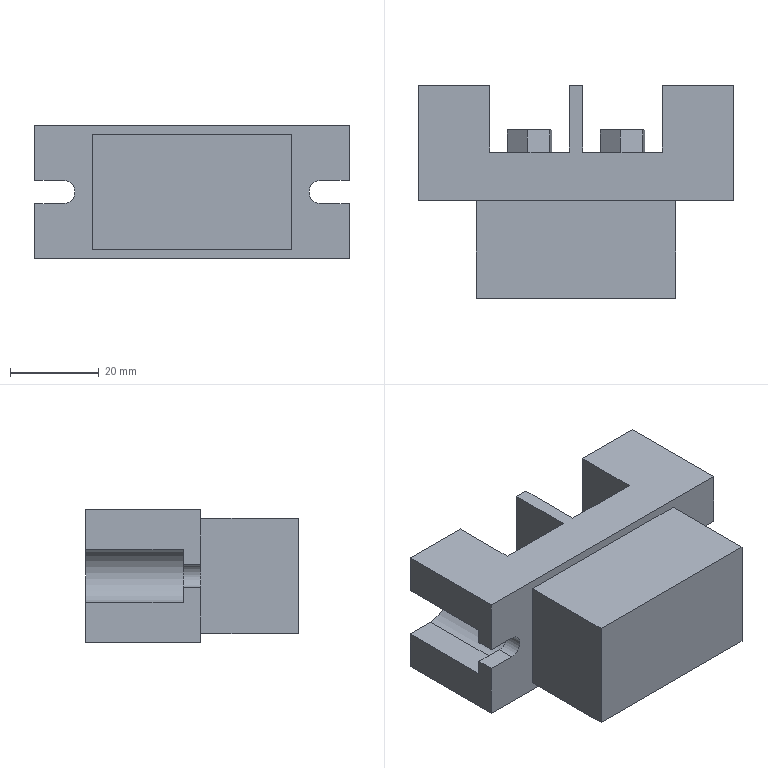Part | SolidWorks | features ICE 5, LPattern 2, Extrusion 1 | 1 solid | 49 faces | box 71 x 48 x 30 mm | volume 59444 mm3 | plane 45 | cylinder 4 | commonest cylinder face diameters 5.2 x2 12 x2
STEP:
#1=CARTESIAN_POINT('',(-19.5,11.,-15.));
#2=VERTEX_POINT('',#1);
#3=CARTESIAN_POINT('',(-19.5,11.,15.));
#4=VERTEX_POINT('',#3);
#5=CARTESIAN_POINT('',(-19.5,11.,-15.));
#6=DIRECTION('',(0.,0.,1.));
#7=VECTOR('',#6,1000.);
#8=LINE('',#5,#7);
#9=EDGE_CURVE('',#2,#4,#8,.T.);
#10=ORIENTED_EDGE('',*,*,#9,.T.);
#11=CARTESIAN_POINT('',(-1.5,11.,15.));
#12=VERTEX_POINT('',#11);
#13=CARTESIAN_POINT('',(-19.5,11.,15.));
#14=DIRECTION('',(1.,0.,0.));
#15=VECTOR('',#14,1000.);
#16=LINE('',#13,#15);
#17=EDGE_CURVE('',#4,#12,#16,.T.);
#18=ORIENTED_EDGE('',*,*,#17,.T.);
#19=CARTESIAN_POINT('',(-1.5,11.,-15.));
#20=VERTEX_POINT('',#19);
#21=CARTESIAN_POINT('',(-1.5,11.,-15.));
#22=DIRECTION('',(0.,0.,-1.));
#23=VECTOR('',#22,1000.);
#24=LINE('',#21,#23);
#25=EDGE_CURVE('',#12,#20,#24,.T.);
#26=ORIENTED_EDGE('',*,*,#25,.T.);
#27=CARTESIAN_POINT('',(-19.5,11.,-15.));
#28=DIRECTION('',(-1.,0.,0.));
#29=VECTOR('',#28,1000.);
#30=LINE('',#27,#29);
#31=EDGE_CURVE('',#20,#2,#30,.T.);
#32=ORIENTED_EDGE('',*,*,#31,.T.);
#33=EDGE_LOOP('',(#10,#18,#26,#32));
#34=FACE_OUTER_BOUND('',#33,.T.);
#35=CARTESIAN_POINT('',(-5.967,11.,3.196));
#36=VERTEX_POINT('',#35);
#37=CARTESIAN_POINT('',(-5.466,11.,-2.328));
#38=VERTEX_POINT('',#37);
#39=CARTESIAN_POINT('',(-5.967,11.,3.196));
#40=DIRECTION('',(0.09034,0.,-0.9959));
#41=VECTOR('',#40,1000.);
#42=LINE('',#39,#41);
#43=EDGE_CURVE('',#36,#38,#42,.T.);
#44=ORIENTED_EDGE('',*,*,#43,.F.);
#45=CARTESIAN_POINT('',(-11.001,11.,5.524));
#46=VERTEX_POINT('',#45);
#47=CARTESIAN_POINT('',(-11.001,11.,5.524));
#48=DIRECTION('',(0.9077,0.,-0.4197));
#49=VECTOR('',#48,1000.);
#50=LINE('',#47,#49);
#51=EDGE_CURVE('',#46,#36,#50,.T.);
#52=ORIENTED_EDGE('',*,*,#51,.F.);
#53=CARTESIAN_POINT('',(-15.534,11.,2.328));
#54=VERTEX_POINT('',#53);
#55=CARTESIAN_POINT('',(-15.534,11.,2.328));
#56=DIRECTION('',(0.8173,0.,0.5762));
#57=VECTOR('',#56,1000.);
#58=LINE('',#55,#57);
#59=EDGE_CURVE('',#54,#46,#58,.T.);
#60=ORIENTED_EDGE('',*,*,#59,.F.);
#61=CARTESIAN_POINT('',(-15.033,11.,-3.196));
#62=VERTEX_POINT('',#61);
#63=CARTESIAN_POINT('',(-15.033,11.,-3.196));
#64=DIRECTION('',(-0.09034,0.,0.9959));
#65=VECTOR('',#64,1000.);
#66=LINE('',#63,#65);
#67=EDGE_CURVE('',#62,#54,#66,.T.);
#68=ORIENTED_EDGE('',*,*,#67,.F.);
#69=CARTESIAN_POINT('',(-9.999,11.,-5.524));
#70=VERTEX_POINT('',#69);
#71=CARTESIAN_POINT('',(-9.999,11.,-5.524));
#72=DIRECTION('',(-0.9077,0.,0.4197));
#73=VECTOR('',#72,1000.);
#74=LINE('',#71,#73);
#75=EDGE_CURVE('',#70,#62,#74,.T.);
#76=ORIENTED_EDGE('',*,*,#75,.F.);
#77=CARTESIAN_POINT('',(-5.466,11.,-2.328));
#78=DIRECTION('',(-0.8173,0.,-0.5762));
#79=VECTOR('',#78,1000.);
#80=LINE('',#77,#79);
#81=EDGE_CURVE('',#38,#70,#80,.T.);
#82=ORIENTED_EDGE('',*,*,#81,.F.);
#83=EDGE_LOOP('',(#44,#52,#60,#68,#76,#82));
#84=FACE_BOUND('',#83,.T.);
#85=CARTESIAN_POINT('',(-21.,11.,0.));
#86=DIRECTION('',(0.,1.,0.));
#87=DIRECTION('',(0.,0.,1.));
#88=AXIS2_PLACEMENT_3D('',#85,#86,#87);
#89=PLANE('',#88);
#90=ADVANCED_FACE('',(#34,#84),#89,.T.);
#91=CARTESIAN_POINT('',(1.5,11.,-15.));
#92=VERTEX_POINT('',#91);
#93=CARTESIAN_POINT('',(1.5,11.,15.));
#94=VERTEX_POINT('',#93);
#95=CARTESIAN_POINT('',(1.5,11.,-15.));
#96=DIRECTION('',(0.,0.,1.));
#97=VECTOR('',#96,1000.);
#98=LINE('',#95,#97);
#99=EDGE_CURVE('',#92,#94,#98,.T.);
#100=ORIENTED_EDGE('',*,*,#99,.T.);
#101=CARTESIAN_POINT('',(19.5,11.,15.));
#102=VERTEX_POINT('',#101);
#103=CARTESIAN_POINT('',(1.5,11.,15.));
#104=DIRECTION('',(1.,0.,0.));
#105=VECTOR('',#104,1000.);
#106=LINE('',#103,#105);
#107=EDGE_CURVE('',#94,#102,#106,.T.);
#108=ORIENTED_EDGE('',*,*,#107,.T.);
#109=CARTESIAN_POINT('',(19.5,11.,-15.));
#110=VERTEX_POINT('',#109);
#111=CARTESIAN_POINT('',(19.5,11.,-15.));
#112=DIRECTION('',(0.,0.,-1.));
#113=VECTOR('',#112,1000.);
#114=LINE('',#111,#113);
#115=EDGE_CURVE('',#102,#110,#114,.T.);
#116=ORIENTED_EDGE('',*,*,#115,.T.);
#117=CARTESIAN_POINT('',(1.5,11.,-15.));
#118=DIRECTION('',(-1.,0.,0.));
#119=VECTOR('',#118,1000.);
#120=LINE('',#117,#119);
#121=EDGE_CURVE('',#110,#92,#120,.T.);
#122=ORIENTED_EDGE('',*,*,#121,.T.);
#123=EDGE_LOOP('',(#100,#108,#116,#122));
#124=FACE_OUTER_BOUND('',#123,.T.);
#125=CARTESIAN_POINT('',(15.033,11.,3.196));
#126=VERTEX_POINT('',#125);
#127=CARTESIAN_POINT('',(15.534,11.,-2.328));
#128=VERTEX_POINT('',#127);
#129=CARTESIAN_POINT('',(15.033,11.,3.196));
#130=DIRECTION('',(0.09034,0.,-0.9959));
#131=VECTOR('',#130,1000.);
#132=LINE('',#129,#131);
#133=EDGE_CURVE('',#126,#128,#132,.T.);
#134=ORIENTED_EDGE('',*,*,#133,.F.);
#135=CARTESIAN_POINT('',(9.999,11.,5.524));
#136=VERTEX_POINT('',#135);
#137=CARTESIAN_POINT('',(9.999,11.,5.524));
#138=DIRECTION('',(0.9077,0.,-0.4197));
#139=VECTOR('',#138,1000.);
#140=LINE('',#137,#139);
#141=EDGE_CURVE('',#136,#126,#140,.T.);
#142=ORIENTED_EDGE('',*,*,#141,.F.);
#143=CARTESIAN_POINT('',(5.466,11.,2.328));
#144=VERTEX_POINT('',#143);
#145=CARTESIAN_POINT('',(5.466,11.,2.328));
#146=DIRECTION('',(0.8173,0.,0.5762));
#147=VECTOR('',#146,1000.);
#148=LINE('',#145,#147);
#149=EDGE_CURVE('',#144,#136,#148,.T.);
#150=ORIENTED_EDGE('',*,*,#149,.F.);
#151=CARTESIAN_POINT('',(5.967,11.,-3.196));
#152=VERTEX_POINT('',#151);
#153=CARTESIAN_POINT('',(5.967,11.,-3.196));
#154=DIRECTION('',(-0.09034,0.,0.9959));
#155=VECTOR('',#154,1000.);
#156=LINE('',#153,#155);
#157=EDGE_CURVE('',#152,#144,#156,.T.);
#158=ORIENTED_EDGE('',*,*,#157,.F.);
#159=CARTESIAN_POINT('',(11.001,11.,-5.524));
#160=VERTEX_POINT('',#159);
#161=CARTESIAN_POINT('',(11.001,11.,-5.524));
#162=DIRECTION('',(-0.9077,0.,0.4197));
#163=VECTOR('',#162,1000.);
#164=LINE('',#161,#163);
#165=EDGE_CURVE('',#160,#152,#164,.T.);
#166=ORIENTED_EDGE('',*,*,#165,.F.);
#167=CARTESIAN_POINT('',(15.534,11.,-2.328));
#168=DIRECTION('',(-0.8173,0.,-0.5762));
#169=VECTOR('',#168,1000.);
#170=LINE('',#167,#169);
#171=EDGE_CURVE('',#128,#160,#170,.T.);
#172=ORIENTED_EDGE('',*,*,#171,.F.);
#173=EDGE_LOOP('',(#134,#142,#150,#158,#166,#172));
#174=FACE_BOUND('',#173,.T.);
#175=CARTESIAN_POINT('',(0.,11.,0.));
#176=DIRECTION('',(0.,1.,0.));
#177=DIRECTION('',(0.,0.,1.));
#178=AXIS2_PLACEMENT_3D('',#175,#176,#177);
#179=PLANE('',#178);
#180=ADVANCED_FACE('',(#124,#174),#179,.T.);
#181=CARTESIAN_POINT('',(-19.5,26.,-15.));
#182=VERTEX_POINT('',#181);
#183=CARTESIAN_POINT('',(-19.5,26.,15.));
#184=VERTEX_POINT('',#183);
#185=CARTESIAN_POINT('',(-19.5,26.,-15.));
#186=DIRECTION('',(0.,0.,1.));
#187=VECTOR('',#186,1000.);
#188=LINE('',#185,#187);
#189=EDGE_CURVE('',#182,#184,#188,.T.);
#190=ORIENTED_EDGE('',*,*,#189,.F.);
#191=CARTESIAN_POINT('',(-35.5,26.,-15.));
#192=VERTEX_POINT('',#191);
#193=CARTESIAN_POINT('',(-35.5,26.,-15.));
#194=DIRECTION('',(-1.,0.,0.));
#195=VECTOR('',#194,1000.);
#196=LINE('',#193,#195);
#197=EDGE_CURVE('',#182,#192,#196,.T.);
#198=ORIENTED_EDGE('',*,*,#197,.T.);
#199=CARTESIAN_POINT('',(-35.5,26.,-6.));
#200=VERTEX_POINT('',#199);
#201=CARTESIAN_POINT('',(-35.5,26.,-15.));
#202=DIRECTION('',(0.,0.,1.));
#203=VECTOR('',#202,1000.);
#204=LINE('',#201,#203);
#205=EDGE_CURVE('',#192,#200,#204,.T.);
#206=ORIENTED_EDGE('',*,*,#205,.T.);
#207=CARTESIAN_POINT('',(-29.,26.,-6.));
#208=VERTEX_POINT('',#207);
#209=CARTESIAN_POINT('',(-29.,26.,-6.));
#210=DIRECTION('',(-1.,0.,0.));
#211=VECTOR('',#210,1000.);
#212=LINE('',#209,#211);
#213=EDGE_CURVE('',#208,#200,#212,.T.);
#214=ORIENTED_EDGE('',*,*,#213,.F.);
#215=CARTESIAN_POINT('',(-29.,26.,6.));
#216=VERTEX_POINT('',#215);
#217=CARTESIAN_POINT('',(-29.,26.,0.));
#218=DIRECTION('',(0.,1.,0.));
#219=DIRECTION('',(0.,0.,1.));
#220=AXIS2_PLACEMENT_3D('',#217,#218,#219);
#221=CIRCLE('',#220,6.);
#222=EDGE_CURVE('',#216,#208,#221,.T.);
#223=ORIENTED_EDGE('',*,*,#222,.F.);
#224=CARTESIAN_POINT('',(-35.5,26.,6.));
#225=VERTEX_POINT('',#224);
#226=CARTESIAN_POINT('',(-29.,26.,6.));
#227=DIRECTION('',(1.,0.,0.));
#228=VECTOR('',#227,1000.);
#229=LINE('',#226,#228);
#230=EDGE_CURVE('',#225,#216,#229,.T.);
#231=ORIENTED_EDGE('',*,*,#230,.F.);
#232=CARTESIAN_POINT('',(-35.5,26.,15.));
#233=VERTEX_POINT('',#232);
#234=CARTESIAN_POINT('',(-35.5,26.,-15.));
#235=DIRECTION('',(0.,0.,1.));
#236=VECTOR('',#235,1000.);
#237=LINE('',#234,#236);
#238=EDGE_CURVE('',#225,#233,#237,.T.);
#239=ORIENTED_EDGE('',*,*,#238,.T.);
#240=CARTESIAN_POINT('',(-35.5,26.,15.));
#241=DIRECTION('',(1.,0.,0.));
#242=VECTOR('',#241,1000.);
#243=LINE('',#240,#242);
#244=EDGE_CURVE('',#233,#184,#243,.T.);
#245=ORIENTED_EDGE('',*,*,#244,.T.);
#246=EDGE_LOOP('',(#190,#198,#206,#214,#223,#231,#239,#245));
#247=FACE_OUTER_BOUND('',#246,.T.);
#248=CARTESIAN_POINT('',(0.,26.,0.));
#249=DIRECTION('',(0.,1.,0.));
#250=DIRECTION('',(0.,0.,1.));
#251=AXIS2_PLACEMENT_3D('',#248,#249,#250);
#252=PLANE('',#251);
#253=ADVANCED_FACE('',(#247),#252,.T.);
#254=CARTESIAN_POINT('',(-1.5,26.,15.));
#255=VERTEX_POINT('',#254);
#256=CARTESIAN_POINT('',(-1.5,26.,-15.));
#257=VERTEX_POINT('',#256);
#258=CARTESIAN_POINT('',(-1.5,26.,-15.));
#259=DIRECTION('',(0.,0.,-1.));
#260=VECTOR('',#259,1000.);
#261=LINE('',#258,#260);
#262=EDGE_CURVE('',#255,#257,#261,.T.);
#263=ORIENTED_EDGE('',*,*,#262,.F.);
#264=CARTESIAN_POINT('',(1.5,26.,15.));
#265=VERTEX_POINT('',#264);
#266=CARTESIAN_POINT('',(-35.5,26.,15.));
#267=DIRECTION('',(1.,0.,0.));
#268=VECTOR('',#267,1000.);
#269=LINE('',#266,#268);
#270=EDGE_CURVE('',#255,#265,#269,.T.);
#271=ORIENTED_EDGE('',*,*,#270,.T.);
#272=CARTESIAN_POINT('',(1.5,26.,-15.));
#273=VERTEX_POINT('',#272);
#274=CARTESIAN_POINT('',(1.5,26.,-15.));
#275=DIRECTION('',(0.,0.,1.));
#276=VECTOR('',#275,1000.);
#277=LINE('',#274,#276);
#278=EDGE_CURVE('',#273,#265,#277,.T.);
#279=ORIENTED_EDGE('',*,*,#278,.F.);
#280=CARTESIAN_POINT('',(-35.5,26.,-15.));
#281=DIRECTION('',(-1.,0.,0.));
#282=VECTOR('',#281,1000.);
#283=LINE('',#280,#282);
#284=EDGE_CURVE('',#273,#257,#283,.T.);
#285=ORIENTED_EDGE('',*,*,#284,.T.);
#286=EDGE_LOOP('',(#263,#271,#279,#285));
#287=FACE_OUTER_BOUND('',#286,.T.);
#288=CARTESIAN_POINT('',(0.,26.,0.));
#289=DIRECTION('',(0.,1.,0.));
#290=DIRECTION('',(0.,0.,1.));
#291=AXIS2_PLACEMENT_3D('',#288,#289,#290);
#292=PLANE('',#291);
#293=ADVANCED_FACE('',(#287),#292,.T.);
#294=CARTESIAN_POINT('',(-29.,4.,-2.6));
#295=VERTEX_POINT('',#294);
#296=CARTESIAN_POINT('',(-29.,4.,2.6));
#297=VERTEX_POINT('',#296);
#298=CARTESIAN_POINT('',(-29.,4.,0.));
#299=DIRECTION('',(0.,-1.,0.));
#300=DIRECTION('',(0.,0.,1.));
#301=AXIS2_PLACEMENT_3D('',#298,#299,#300);
#302=CIRCLE('',#301,2.6);
#303=EDGE_CURVE('',#295,#297,#302,.T.);
#304=ORIENTED_EDGE('',*,*,#303,.F.);
#305=CARTESIAN_POINT('',(-29.,0.,-2.6));
#306=VERTEX_POINT('',#305);
#307=CARTESIAN_POINT('',(-29.,-22.,-2.6));
#308=DIRECTION('',(0.,1.,0.));
#309=VECTOR('',#308,1000.);
#310=LINE('',#307,#309);
#311=EDGE_CURVE('',#306,#295,#310,.T.);
#312=ORIENTED_EDGE('',*,*,#311,.F.);
#313=CARTESIAN_POINT('',(-29.,0.,2.6));
#314=VERTEX_POINT('',#313);
#315=CARTESIAN_POINT('',(-29.,0.,0.));
#316=DIRECTION('',(0.,1.,0.));
#317=DIRECTION('',(0.,0.,1.));
#318=AXIS2_PLACEMENT_3D('',#315,#316,#317);
#319=CIRCLE('',#318,2.6);
#320=EDGE_CURVE('',#314,#306,#319,.T.);
#321=ORIENTED_EDGE('',*,*,#320,.F.);
#322=CARTESIAN_POINT('',(-29.,-22.,2.6));
#323=DIRECTION('',(0.,1.,0.));
#324=VECTOR('',#323,1000.);
#325=LINE('',#322,#324);
#326=EDGE_CURVE('',#314,#297,#325,.T.);
#327=ORIENTED_EDGE('',*,*,#326,.T.);
#328=EDGE_LOOP('',(#304,#312,#321,#327));
#329=FACE_OUTER_BOUND('',#328,.T.);
#330=CARTESIAN_POINT('',(-29.,-22.,0.));
#331=DIRECTION('',(0.,1.,0.));
#332=DIRECTION('',(0.,0.,1.));
#333=AXIS2_PLACEMENT_3D('',#330,#331,#332);
#334=CYLINDRICAL_SURFACE('',#333,2.6);
#335=ADVANCED_FACE('',(#329),#334,.F.);
#336=CARTESIAN_POINT('',(-35.5,4.,2.6));
#337=VERTEX_POINT('',#336);
#338=CARTESIAN_POINT('',(-29.,4.,2.6));
#339=DIRECTION('',(-1.,0.,0.));
#340=VECTOR('',#339,1000.);
#341=LINE('',#338,#340);
#342=EDGE_CURVE('',#297,#337,#341,.T.);
#343=ORIENTED_EDGE('',*,*,#342,.F.);
#344=ORIENTED_EDGE('',*,*,#326,.F.);
#345=CARTESIAN_POINT('',(-35.5,0.,2.6));
#346=VERTEX_POINT('',#345);
#347=CARTESIAN_POINT('',(0.,0.,2.6));
#348=DIRECTION('',(1.,0.,0.));
#349=VECTOR('',#348,1000.);
#350=LINE('',#347,#349);
#351=EDGE_CURVE('',#346,#314,#350,.T.);
#352=ORIENTED_EDGE('',*,*,#351,.F.);
#353=CARTESIAN_POINT('',(-35.5,26.,2.6));
#354=DIRECTION('',(0.,-1.,0.));
#355=VECTOR('',#354,1000.);
#356=LINE('',#353,#355);
#357=EDGE_CURVE('',#337,#346,#356,.T.);
#358=ORIENTED_EDGE('',*,*,#357,.F.);
#359=EDGE_LOOP('',(#343,#344,#352,#358));
#360=FACE_OUTER_BOUND('',#359,.T.);
#361=CARTESIAN_POINT('',(-29.,-22.,2.6));
#362=DIRECTION('',(0.,0.,1.));
#363=DIRECTION('',(1.,0.,0.));
#364=AXIS2_PLACEMENT_3D('',#361,#362,#363);
#365=PLANE('',#364);
#366=ADVANCED_FACE('',(#360),#365,.F.);
#367=CARTESIAN_POINT('',(-35.5,4.,-2.6));
#368=VERTEX_POINT('',#367);
#369=CARTESIAN_POINT('',(-29.,4.,-2.6));
#370=DIRECTION('',(1.,0.,0.));
#371=VECTOR('',#370,1000.);
#372=LINE('',#369,#371);
#373=EDGE_CURVE('',#368,#295,#372,.T.);
#374=ORIENTED_EDGE('',*,*,#373,.F.);
#375=CARTESIAN_POINT('',(-35.5,0.,-2.6));
#376=VERTEX_POINT('',#375);
#377=CARTESIAN_POINT('',(-35.5,26.,-2.6));
#378=DIRECTION('',(0.,1.,0.));
#379=VECTOR('',#378,1000.);
#380=LINE('',#377,#379);
#381=EDGE_CURVE('',#376,#368,#380,.T.);
#382=ORIENTED_EDGE('',*,*,#381,.F.);
#383=CARTESIAN_POINT('',(0.,0.,-2.6));
#384=DIRECTION('',(-1.,0.,0.));
#385=VECTOR('',#384,1000.);
#386=LINE('',#383,#385);
#387=EDGE_CURVE('',#306,#376,#386,.T.);
#388=ORIENTED_EDGE('',*,*,#387,.F.);
#389=ORIENTED_EDGE('',*,*,#311,.T.);
#390=EDGE_LOOP('',(#374,#382,#388,#389));
#391=FACE_OUTER_BOUND('',#390,.T.);
#392=CARTESIAN_POINT('',(-29.,-22.,-2.6));
#393=DIRECTION('',(0.,0.,-1.));
#394=DIRECTION('',(-1.,0.,0.));
#395=AXIS2_PLACEMENT_3D('',#392,#393,#394);
#396=PLANE('',#395);
#397=ADVANCED_FACE('',(#391),#396,.F.);
#398=CARTESIAN_POINT('',(29.,4.,2.6));
#399=VERTEX_POINT('',#398);
#400=CARTESIAN_POINT('',(29.,4.,-2.6));
#401=VERTEX_POINT('',#400);
#402=CARTESIAN_POINT('',(29.,4.,0.));
#403=DIRECTION('',(0.,-1.,0.));
#404=DIRECTION('',(0.,0.,1.));
#405=AXIS2_PLACEMENT_3D('',#402,#403,#404);
#406=CIRCLE('',#405,2.6);
#407=EDGE_CURVE('',#399,#401,#406,.T.);
#408=ORIENTED_EDGE('',*,*,#407,.F.);
#409=CARTESIAN_POINT('',(29.,0.,2.6));
#410=VERTEX_POINT('',#409);
#411=CARTESIAN_POINT('',(29.,-22.,2.6));
#412=DIRECTION('',(0.,1.,0.));
#413=VECTOR('',#412,1000.);
#414=LINE('',#411,#413);
#415=EDGE_CURVE('',#410,#399,#414,.T.);
#416=ORIENTED_EDGE('',*,*,#415,.F.);
#417=CARTESIAN_POINT('',(29.,0.,-2.6));
#418=VERTEX_POINT('',#417);
#419=CARTESIAN_POINT('',(29.,0.,0.));
#420=DIRECTION('',(0.,1.,0.));
#421=DIRECTION('',(0.,0.,1.));
#422=AXIS2_PLACEMENT_3D('',#419,#420,#421);
#423=CIRCLE('',#422,2.6);
#424=EDGE_CURVE('',#418,#410,#423,.T.);
#425=ORIENTED_EDGE('',*,*,#424,.F.);
#426=CARTESIAN_POINT('',(29.,-22.,-2.6));
#427=DIRECTION('',(0.,1.,0.));
#428=VECTOR('',#427,1000.);
#429=LINE('',#426,#428);
#430=EDGE_CURVE('',#418,#401,#429,.T.);
#431=ORIENTED_EDGE('',*,*,#430,.T.);
#432=EDGE_LOOP('',(#408,#416,#425,#431));
#433=FACE_OUTER_BOUND('',#432,.T.);
#434=CARTESIAN_POINT('',(29.,-22.,0.));
#435=DIRECTION('',(0.,1.,0.));
#436=DIRECTION('',(0.,0.,1.));
#437=AXIS2_PLACEMENT_3D('',#434,#435,#436);
#438=CYLINDRICAL_SURFACE('',#437,2.6);
#439=ADVANCED_FACE('',(#433),#438,.F.);
#440=CARTESIAN_POINT('',(35.5,4.,-2.6));
#441=VERTEX_POINT('',#440);
#442=CARTESIAN_POINT('',(29.,4.,-2.6));
#443=DIRECTION('',(1.,0.,0.));
#444=VECTOR('',#443,1000.);
#445=LINE('',#442,#444);
#446=EDGE_CURVE('',#401,#441,#445,.T.);
#447=ORIENTED_EDGE('',*,*,#446,.F.);
#448=ORIENTED_EDGE('',*,*,#430,.F.);
#449=CARTESIAN_POINT('',(35.5,0.,-2.6));
#450=VERTEX_POINT('',#449);
#451=CARTESIAN_POINT('',(0.,0.,-2.6));
#452=DIRECTION('',(-1.,0.,0.));
#453=VECTOR('',#452,1000.);
#454=LINE('',#451,#453);
#455=EDGE_CURVE('',#450,#418,#454,.T.);
#456=ORIENTED_EDGE('',*,*,#455,.F.);
#457=CARTESIAN_POINT('',(35.5,26.,-2.6));
#458=DIRECTION('',(0.,-1.,0.));
#459=VECTOR('',#458,1000.);
#460=LINE('',#457,#459);
#461=EDGE_CURVE('',#441,#450,#460,.T.);
#462=ORIENTED_EDGE('',*,*,#461,.F.);
#463=EDGE_LOOP('',(#447,#448,#456,#462));
#464=FACE_OUTER_BOUND('',#463,.T.);
#465=CARTESIAN_POINT('',(29.,-22.,-2.6));
#466=DIRECTION('',(0.,0.,-1.));
#467=DIRECTION('',(-1.,0.,0.));
#468=AXIS2_PLACEMENT_3D('',#465,#466,#467);
#469=PLANE('',#468);
#470=ADVANCED_FACE('',(#464),#469,.F.);
#471=CARTESIAN_POINT('',(35.5,4.,2.6));
#472=VERTEX_POINT('',#471);
#473=CARTESIAN_POINT('',(29.,4.,2.6));
#474=DIRECTION('',(-1.,0.,0.));
#475=VECTOR('',#474,1000.);
#476=LINE('',#473,#475);
#477=EDGE_CURVE('',#472,#399,#476,.T.);
#478=ORIENTED_EDGE('',*,*,#477,.F.);
#479=CARTESIAN_POINT('',(35.5,0.,2.6));
#480=VERTEX_POINT('',#479);
#481=CARTESIAN_POINT('',(35.5,26.,2.6));
#482=DIRECTION('',(0.,1.,0.));
#483=VECTOR('',#482,1000.);
#484=LINE('',#481,#483);
#485=EDGE_CURVE('',#480,#472,#484,.T.);
#486=ORIENTED_EDGE('',*,*,#485,.F.);
#487=CARTESIAN_POINT('',(0.,0.,2.6));
#488=DIRECTION('',(1.,0.,0.));
#489=VECTOR('',#488,1000.);
#490=LINE('',#487,#489);
#491=EDGE_CURVE('',#410,#480,#490,.T.);
#492=ORIENTED_EDGE('',*,*,#491,.F.);
#493=ORIENTED_EDGE('',*,*,#415,.T.);
#494=EDGE_LOOP('',(#478,#486,#492,#493));
#495=FACE_OUTER_BOUND('',#494,.T.);
#496=CARTESIAN_POINT('',(29.,-22.,2.6));
#497=DIRECTION('',(0.,0.,1.));
#498=DIRECTION('',(1.,0.,0.));
#499=AXIS2_PLACEMENT_3D('',#496,#497,#498);
#500=PLANE('',#499);
#501=ADVANCED_FACE('',(#495),#500,.F.);
#502=CARTESIAN_POINT('',(35.5,26.,-6.));
#503=VERTEX_POINT('',#502);
#504=CARTESIAN_POINT('',(35.5,26.,-15.));
#505=VERTEX_POINT('',#504);
#506=CARTESIAN_POINT('',(35.5,26.,-15.));
#507=DIRECTION('',(0.,0.,-1.));
#508=VECTOR('',#507,1000.);
#509=LINE('',#506,#508);
#510=EDGE_CURVE('',#503,#505,#509,.T.);
#511=ORIENTED_EDGE('',*,*,#510,.F.);
#512=CARTESIAN_POINT('',(35.5,4.,-6.));
#513=VERTEX_POINT('',#512);
#514=CARTESIAN_POINT('',(35.5,26.,-6.));
#515=DIRECTION('',(0.,-1.,0.));
#516=VECTOR('',#515,1000.);
#517=LINE('',#514,#516);
#518=EDGE_CURVE('',#503,#513,#517,.T.);
#519=ORIENTED_EDGE('',*,*,#518,.T.);
#520=CARTESIAN_POINT('',(35.5,4.,-15.));
#521=DIRECTION('',(0.,0.,-1.));
#522=VECTOR('',#521,1000.);
#523=LINE('',#520,#522);
#524=EDGE_CURVE('',#441,#513,#523,.T.);
#525=ORIENTED_EDGE('',*,*,#524,.F.);
#526=ORIENTED_EDGE('',*,*,#461,.T.);
#527=CARTESIAN_POINT('',(35.5,0.,-15.));
#528=VERTEX_POINT('',#527);
#529=CARTESIAN_POINT('',(35.5,0.,-15.));
#530=DIRECTION('',(0.,0.,-1.));
#531=VECTOR('',#530,1000.);
#532=LINE('',#529,#531);
#533=EDGE_CURVE('',#450,#528,#532,.T.);
#534=ORIENTED_EDGE('',*,*,#533,.T.);
#535=CARTESIAN_POINT('',(35.5,26.,-15.));
#536=DIRECTION('',(0.,-1.,0.));
#537=VECTOR('',#536,1000.);
#538=LINE('',#535,#537);
#539=EDGE_CURVE('',#505,#528,#538,.T.);
#540=ORIENTED_EDGE('',*,*,#539,.F.);
#541=EDGE_LOOP('',(#511,#519,#525,#526,#534,#540));
#542=FACE_OUTER_BOUND('',#541,.T.);
#543=CARTESIAN_POINT('',(35.5,26.,-15.));
#544=DIRECTION('',(-1.,0.,0.));
#545=DIRECTION('',(0.,0.,1.));
#546=AXIS2_PLACEMENT_3D('',#543,#544,#545);
#547=PLANE('',#546);
#548=ADVANCED_FACE('',(#542),#547,.F.);
#549=ORIENTED_EDGE('',*,*,#238,.F.);
#550=CARTESIAN_POINT('',(-35.5,4.,6.));
#551=VERTEX_POINT('',#550);
#552=CARTESIAN_POINT('',(-35.5,26.,6.));
#553=DIRECTION('',(0.,-1.,0.));
#554=VECTOR('',#553,1000.);
#555=LINE('',#552,#554);
#556=EDGE_CURVE('',#225,#551,#555,.T.);
#557=ORIENTED_EDGE('',*,*,#556,.T.);
#558=CARTESIAN_POINT('',(-35.5,4.,-15.));
#559=DIRECTION('',(0.,0.,1.));
#560=VECTOR('',#559,1000.);
#561=LINE('',#558,#560);
#562=EDGE_CURVE('',#337,#551,#561,.T.);
#563=ORIENTED_EDGE('',*,*,#562,.F.);
#564=ORIENTED_EDGE('',*,*,#357,.T.);
#565=CARTESIAN_POINT('',(-35.5,0.,15.));
#566=VERTEX_POINT('',#565);
#567=CARTESIAN_POINT('',(-35.5,0.,-15.));
#568=DIRECTION('',(0.,0.,1.));
#569=VECTOR('',#568,1000.);
#570=LINE('',#567,#569);
#571=EDGE_CURVE('',#346,#566,#570,.T.);
#572=ORIENTED_EDGE('',*,*,#571,.T.);
#573=CARTESIAN_POINT('',(-35.5,26.,15.));
#574=DIRECTION('',(0.,-1.,0.));
#575=VECTOR('',#574,1000.);
#576=LINE('',#573,#575);
#577=EDGE_CURVE('',#233,#566,#576,.T.);
#578=ORIENTED_EDGE('',*,*,#577,.F.);
#579=EDGE_LOOP('',(#549,#557,#563,#564,#572,#578));
#580=FACE_OUTER_BOUND('',#579,.T.);
#581=CARTESIAN_POINT('',(-35.5,26.,-15.));
#582=DIRECTION('',(1.,0.,0.));
#583=DIRECTION('',(0.,0.,-1.));
#584=AXIS2_PLACEMENT_3D('',#581,#582,#583);
#585=PLANE('',#584);
#586=ADVANCED_FACE('',(#580),#585,.F.);
#587=ORIENTED_EDGE('',*,*,#533,.F.);
#588=ORIENTED_EDGE('',*,*,#455,.T.);
#589=ORIENTED_EDGE('',*,*,#424,.T.);
#590=ORIENTED_EDGE('',*,*,#491,.T.);
#591=CARTESIAN_POINT('',(35.5,0.,15.));
#592=VERTEX_POINT('',#591);
#593=CARTESIAN_POINT('',(35.5,0.,-15.));
#594=DIRECTION('',(0.,0.,-1.));
#595=VECTOR('',#594,1000.);
#596=LINE('',#593,#595);
#597=EDGE_CURVE('',#592,#480,#596,.T.);
#598=ORIENTED_EDGE('',*,*,#597,.F.);
#599=CARTESIAN_POINT('',(-35.5,0.,15.));
#600=DIRECTION('',(1.,0.,0.));
#601=VECTOR('',#600,1000.);
#602=LINE('',#599,#601);
#603=EDGE_CURVE('',#566,#592,#602,.T.);
#604=ORIENTED_EDGE('',*,*,#603,.F.);
#605=ORIENTED_EDGE('',*,*,#571,.F.);
#606=ORIENTED_EDGE('',*,*,#351,.T.);
#607=ORIENTED_EDGE('',*,*,#320,.T.);
#608=ORIENTED_EDGE('',*,*,#387,.T.);
#609=CARTESIAN_POINT('',(-35.5,0.,-15.));
#610=VERTEX_POINT('',#609);
#611=CARTESIAN_POINT('',(-35.5,0.,-15.));
#612=DIRECTION('',(0.,0.,1.));
#613=VECTOR('',#612,1000.);
#614=LINE('',#611,#613);
#615=EDGE_CURVE('',#610,#376,#614,.T.);
#616=ORIENTED_EDGE('',*,*,#615,.F.);
#617=CARTESIAN_POINT('',(-35.5,0.,-15.));
#618=DIRECTION('',(-1.,0.,0.));
#619=VECTOR('',#618,1000.);
#620=LINE('',#617,#619);
#621=EDGE_CURVE('',#528,#610,#620,.T.);
#622=ORIENTED_EDGE('',*,*,#621,.F.);
#623=EDGE_LOOP('',(#587,#588,#589,#590,#598,#604,#605,#606,#607,#608,#616,#622));
#624=FACE_OUTER_BOUND('',#623,.T.);
#625=CARTESIAN_POINT('',(22.5,0.,-13.));
#626=VERTEX_POINT('',#625);
#627=CARTESIAN_POINT('',(22.5,0.,13.));
#628=VERTEX_POINT('',#627);
#629=CARTESIAN_POINT('',(22.5,0.,13.));
#630=DIRECTION('',(0.,0.,1.));
#631=VECTOR('',#630,1000.);
#632=LINE('',#629,#631);
#633=EDGE_CURVE('',#626,#628,#632,.T.);
#634=ORIENTED_EDGE('',*,*,#633,.F.);
#635=CARTESIAN_POINT('',(-22.5,0.,-13.));
#636=VERTEX_POINT('',#635);
#637=CARTESIAN_POINT('',(-22.5,0.,-13.));
#638=DIRECTION('',(1.,0.,0.));
#639=VECTOR('',#638,1000.);
#640=LINE('',#637,#639);
#641=EDGE_CURVE('',#636,#626,#640,.T.);
#642=ORIENTED_EDGE('',*,*,#641,.F.);
#643=CARTESIAN_POINT('',(-22.5,0.,13.));
#644=VERTEX_POINT('',#643);
#645=CARTESIAN_POINT('',(-22.5,0.,13.));
#646=DIRECTION('',(0.,0.,-1.));
#647=VECTOR('',#646,1000.);
#648=LINE('',#645,#647);
#649=EDGE_CURVE('',#644,#636,#648,.T.);
#650=ORIENTED_EDGE('',*,*,#649,.F.);
#651=CARTESIAN_POINT('',(-22.5,0.,13.));
#652=DIRECTION('',(-1.,0.,0.));
#653=VECTOR('',#652,1000.);
#654=LINE('',#651,#653);
#655=EDGE_CURVE('',#628,#644,#654,.T.);
#656=ORIENTED_EDGE('',*,*,#655,.F.);
#657=EDGE_LOOP('',(#634,#642,#650,#656));
#658=FACE_BOUND('',#657,.T.);
#659=CARTESIAN_POINT('',(0.,0.,0.));
#660=DIRECTION('',(0.,1.,0.));
#661=DIRECTION('',(0.,0.,1.));
#662=AXIS2_PLACEMENT_3D('',#659,#660,#661);
#663=PLANE('',#662);
#664=ADVANCED_FACE('',(#624,#658),#663,.F.);
#665=CARTESIAN_POINT('',(35.5,4.,6.));
#666=VERTEX_POINT('',#665);
#667=CARTESIAN_POINT('',(35.5,4.,-15.));
#668=DIRECTION('',(0.,0.,-1.));
#669=VECTOR('',#668,1000.);
#670=LINE('',#667,#669);
#671=EDGE_CURVE('',#666,#472,#670,.T.);
#672=ORIENTED_EDGE('',*,*,#671,.F.);
#673=CARTESIAN_POINT('',(35.5,26.,6.));
#674=VERTEX_POINT('',#673);
#675=CARTESIAN_POINT('',(35.5,26.,6.));
#676=DIRECTION('',(0.,1.,0.));
#677=VECTOR('',#676,1000.);
#678=LINE('',#675,#677);
#679=EDGE_CURVE('',#666,#674,#678,.T.);
#680=ORIENTED_EDGE('',*,*,#679,.T.);
#681=CARTESIAN_POINT('',(35.5,26.,15.));
#682=VERTEX_POINT('',#681);
#683=CARTESIAN_POINT('',(35.5,26.,-15.));
#684=DIRECTION('',(0.,0.,-1.));
#685=VECTOR('',#684,1000.);
#686=LINE('',#683,#685);
#687=EDGE_CURVE('',#682,#674,#686,.T.);
#688=ORIENTED_EDGE('',*,*,#687,.F.);
#689=CARTESIAN_POINT('',(35.5,26.,15.));
#690=DIRECTION('',(0.,-1.,0.));
#691=VECTOR('',#690,1000.);
#692=LINE('',#689,#691);
#693=EDGE_CURVE('',#682,#592,#692,.T.);
#694=ORIENTED_EDGE('',*,*,#693,.T.);
#695=ORIENTED_EDGE('',*,*,#597,.T.);
#696=ORIENTED_EDGE('',*,*,#485,.T.);
#697=EDGE_LOOP('',(#672,#680,#688,#694,#695,#696));
#698=FACE_OUTER_BOUND('',#697,.T.);
#699=CARTESIAN_POINT('',(35.5,26.,-15.));
#700=DIRECTION('',(-1.,0.,0.));
#701=DIRECTION('',(0.,0.,1.));
#702=AXIS2_PLACEMENT_3D('',#699,#700,#701);
#703=PLANE('',#702);
#704=ADVANCED_FACE('',(#698),#703,.F.);
#705=ORIENTED_EDGE('',*,*,#197,.F.);
#706=CARTESIAN_POINT('',(-19.5,11.,-15.));
#707=DIRECTION('',(0.,1.,0.));
#708=VECTOR('',#707,1000.);
#709=LINE('',#706,#708);
#710=EDGE_CURVE('',#2,#182,#709,.T.);
#711=ORIENTED_EDGE('',*,*,#710,.F.);
#712=ORIENTED_EDGE('',*,*,#31,.F.);
#713=CARTESIAN_POINT('',(-1.5,11.,-15.));
#714=DIRECTION('',(0.,1.,0.));
#715=VECTOR('',#714,1000.);
#716=LINE('',#713,#715);
#717=EDGE_CURVE('',#20,#257,#716,.T.);
#718=ORIENTED_EDGE('',*,*,#717,.T.);
#719=ORIENTED_EDGE('',*,*,#284,.F.);
#720=CARTESIAN_POINT('',(1.5,11.,-15.));
#721=DIRECTION('',(0.,1.,0.));
#722=VECTOR('',#721,1000.);
#723=LINE('',#720,#722);
#724=EDGE_CURVE('',#92,#273,#723,.T.);
#725=ORIENTED_EDGE('',*,*,#724,.F.);
#726=ORIENTED_EDGE('',*,*,#121,.F.);
#727=CARTESIAN_POINT('',(19.5,26.,-15.));
#728=VERTEX_POINT('',#727);
#729=CARTESIAN_POINT('',(19.5,11.,-15.));
#730=DIRECTION('',(0.,1.,0.));
#731=VECTOR('',#730,1000.);
#732=LINE('',#729,#731);
#733=EDGE_CURVE('',#110,#728,#732,.T.);
#734=ORIENTED_EDGE('',*,*,#733,.T.);
#735=CARTESIAN_POINT('',(-35.5,26.,-15.));
#736=DIRECTION('',(-1.,0.,0.));
#737=VECTOR('',#736,1000.);
#738=LINE('',#735,#737);
#739=EDGE_CURVE('',#505,#728,#738,.T.);
#740=ORIENTED_EDGE('',*,*,#739,.F.);
#741=ORIENTED_EDGE('',*,*,#539,.T.);
#742=ORIENTED_EDGE('',*,*,#621,.T.);
#743=CARTESIAN_POINT('',(-35.5,26.,-15.));
#744=DIRECTION('',(0.,-1.,0.));
#745=VECTOR('',#744,1000.);
#746=LINE('',#743,#745);
#747=EDGE_CURVE('',#192,#610,#746,.T.);
#748=ORIENTED_EDGE('',*,*,#747,.F.);
#749=EDGE_LOOP('',(#705,#711,#712,#718,#719,#725,#726,#734,#740,#741,#742,#748));
#750=FACE_OUTER_BOUND('',#749,.T.);
#751=CARTESIAN_POINT('',(-35.5,26.,-15.));
#752=DIRECTION('',(0.,0.,1.));
#753=DIRECTION('',(1.,0.,0.));
#754=AXIS2_PLACEMENT_3D('',#751,#752,#753);
#755=PLANE('',#754);
#756=ADVANCED_FACE('',(#750),#755,.F.);
#757=CARTESIAN_POINT('',(-35.5,4.,-6.));
#758=VERTEX_POINT('',#757);
#759=CARTESIAN_POINT('',(-35.5,4.,-15.));
#760=DIRECTION('',(0.,0.,1.));
#761=VECTOR('',#760,1000.);
#762=LINE('',#759,#761);
#763=EDGE_CURVE('',#758,#368,#762,.T.);
#764=ORIENTED_EDGE('',*,*,#763,.F.);
#765=CARTESIAN_POINT('',(-35.5,26.,-6.));
#766=DIRECTION('',(0.,1.,0.));
#767=VECTOR('',#766,1000.);
#768=LINE('',#765,#767);
#769=EDGE_CURVE('',#758,#200,#768,.T.);
#770=ORIENTED_EDGE('',*,*,#769,.T.);
#771=ORIENTED_EDGE('',*,*,#205,.F.);
#772=ORIENTED_EDGE('',*,*,#747,.T.);
#773=ORIENTED_EDGE('',*,*,#615,.T.);
#774=ORIENTED_EDGE('',*,*,#381,.T.);
#775=EDGE_LOOP('',(#764,#770,#771,#772,#773,#774));
#776=FACE_OUTER_BOUND('',#775,.T.);
#777=CARTESIAN_POINT('',(-35.5,26.,-15.));
#778=DIRECTION('',(1.,0.,0.));
#779=DIRECTION('',(0.,0.,-1.));
#780=AXIS2_PLACEMENT_3D('',#777,#778,#779);
#781=PLANE('',#780);
#782=ADVANCED_FACE('',(#776),#781,.F.);
#783=ORIENTED_EDGE('',*,*,#17,.F.);
#784=CARTESIAN_POINT('',(-19.5,11.,15.));
#785=DIRECTION('',(0.,1.,0.));
#786=VECTOR('',#785,1000.);
#787=LINE('',#784,#786);
#788=EDGE_CURVE('',#4,#184,#787,.T.);
#789=ORIENTED_EDGE('',*,*,#788,.T.);
#790=ORIENTED_EDGE('',*,*,#244,.F.);
#791=ORIENTED_EDGE('',*,*,#577,.T.);
#792=ORIENTED_EDGE('',*,*,#603,.T.);
#793=ORIENTED_EDGE('',*,*,#693,.F.);
#794=CARTESIAN_POINT('',(19.5,26.,15.));
#795=VERTEX_POINT('',#794);
#796=CARTESIAN_POINT('',(-35.5,26.,15.));
#797=DIRECTION('',(1.,0.,0.));
#798=VECTOR('',#797,1000.);
#799=LINE('',#796,#798);
#800=EDGE_CURVE('',#795,#682,#799,.T.);
#801=ORIENTED_EDGE('',*,*,#800,.F.);
#802=CARTESIAN_POINT('',(19.5,11.,15.));
#803=DIRECTION('',(0.,1.,0.));
#804=VECTOR('',#803,1000.);
#805=LINE('',#802,#804);
#806=EDGE_CURVE('',#102,#795,#805,.T.);
#807=ORIENTED_EDGE('',*,*,#806,.F.);
#808=ORIENTED_EDGE('',*,*,#107,.F.);
#809=CARTESIAN_POINT('',(1.5,11.,15.));
#810=DIRECTION('',(0.,1.,0.));
#811=VECTOR('',#810,1000.);
#812=LINE('',#809,#811);
#813=EDGE_CURVE('',#94,#265,#812,.T.);
#814=ORIENTED_EDGE('',*,*,#813,.T.);
#815=ORIENTED_EDGE('',*,*,#270,.F.);
#816=CARTESIAN_POINT('',(-1.5,11.,15.));
#817=DIRECTION('',(0.,1.,0.));
#818=VECTOR('',#817,1000.);
#819=LINE('',#816,#818);
#820=EDGE_CURVE('',#12,#255,#819,.T.);
#821=ORIENTED_EDGE('',*,*,#820,.F.);
#822=EDGE_LOOP('',(#783,#789,#790,#791,#792,#793,#801,#807,#808,#814,#815,#821));
#823=FACE_OUTER_BOUND('',#822,.T.);
#824=CARTESIAN_POINT('',(-35.5,26.,15.));
#825=DIRECTION('',(0.,0.,-1.));
#826=DIRECTION('',(-1.,0.,0.));
#827=AXIS2_PLACEMENT_3D('',#824,#825,#826);
#828=PLANE('',#827);
#829=ADVANCED_FACE('',(#823),#828,.F.);
#830=CARTESIAN_POINT('',(19.5,26.,-15.));
#831=DIRECTION('',(0.,0.,-1.));
#832=VECTOR('',#831,1000.);
#833=LINE('',#830,#832);
#834=EDGE_CURVE('',#795,#728,#833,.T.);
#835=ORIENTED_EDGE('',*,*,#834,.F.);
#836=ORIENTED_EDGE('',*,*,#800,.T.);
#837=ORIENTED_EDGE('',*,*,#687,.T.);
#838=CARTESIAN_POINT('',(29.,26.,6.));
#839=VERTEX_POINT('',#838);
#840=CARTESIAN_POINT('',(29.,26.,6.));
#841=DIRECTION('',(1.,0.,0.));
#842=VECTOR('',#841,1000.);
#843=LINE('',#840,#842);
#844=EDGE_CURVE('',#839,#674,#843,.T.);
#845=ORIENTED_EDGE('',*,*,#844,.F.);
#846=CARTESIAN_POINT('',(29.,26.,-6.));
#847=VERTEX_POINT('',#846);
#848=CARTESIAN_POINT('',(29.,26.,0.));
#849=DIRECTION('',(0.,1.,0.));
#850=DIRECTION('',(0.,0.,1.));
#851=AXIS2_PLACEMENT_3D('',#848,#849,#850);
#852=CIRCLE('',#851,6.);
#853=EDGE_CURVE('',#847,#839,#852,.T.);
#854=ORIENTED_EDGE('',*,*,#853,.F.);
#855=CARTESIAN_POINT('',(29.,26.,-6.));
#856=DIRECTION('',(-1.,0.,0.));
#857=VECTOR('',#856,1000.);
#858=LINE('',#855,#857);
#859=EDGE_CURVE('',#503,#847,#858,.T.);
#860=ORIENTED_EDGE('',*,*,#859,.F.);
#861=ORIENTED_EDGE('',*,*,#510,.T.);
#862=ORIENTED_EDGE('',*,*,#739,.T.);
#863=EDGE_LOOP('',(#835,#836,#837,#845,#854,#860,#861,#862));
#864=FACE_OUTER_BOUND('',#863,.T.);
#865=CARTESIAN_POINT('',(0.,26.,0.));
#866=DIRECTION('',(0.,1.,0.));
#867=DIRECTION('',(0.,0.,1.));
#868=AXIS2_PLACEMENT_3D('',#865,#866,#867);
#869=PLANE('',#868);
#870=ADVANCED_FACE('',(#864),#869,.T.);
#871=ORIENTED_EDGE('',*,*,#633,.T.);
#872=CARTESIAN_POINT('',(22.5,-22.,13.));
#873=VERTEX_POINT('',#872);
#874=CARTESIAN_POINT('',(22.5,-22.,13.));
#875=DIRECTION('',(0.,1.,0.));
#876=VECTOR('',#875,1000.);
#877=LINE('',#874,#876);
#878=EDGE_CURVE('',#873,#628,#877,.T.);
#879=ORIENTED_EDGE('',*,*,#878,.F.);
#880=CARTESIAN_POINT('',(22.5,-22.,-13.));
#881=VERTEX_POINT('',#880);
#882=CARTESIAN_POINT('',(22.5,-22.,13.));
#883=DIRECTION('',(0.,0.,1.));
#884=VECTOR('',#883,1000.);
#885=LINE('',#882,#884);
#886=EDGE_CURVE('',#881,#873,#885,.T.);
#887=ORIENTED_EDGE('',*,*,#886,.F.);
#888=CARTESIAN_POINT('',(22.5,-22.,-13.));
#889=DIRECTION('',(0.,1.,0.));
#890=VECTOR('',#889,1000.);
#891=LINE('',#888,#890);
#892=EDGE_CURVE('',#881,#626,#891,.T.);
#893=ORIENTED_EDGE('',*,*,#892,.T.);
#894=EDGE_LOOP('',(#871,#879,#887,#893));
#895=FACE_OUTER_BOUND('',#894,.T.);
#896=CARTESIAN_POINT('',(22.5,-22.,13.));
#897=DIRECTION('',(-1.,0.,0.));
#898=DIRECTION('',(0.,0.,1.));
#899=AXIS2_PLACEMENT_3D('',#896,#897,#898);
#900=PLANE('',#899);
#901=ADVANCED_FACE('',(#895),#900,.F.);
#902=ORIENTED_EDGE('',*,*,#655,.T.);
#903=CARTESIAN_POINT('',(-22.5,-22.,13.));
#904=VERTEX_POINT('',#903);
#905=CARTESIAN_POINT('',(-22.5,-22.,13.));
#906=DIRECTION('',(0.,1.,0.));
#907=VECTOR('',#906,1000.);
#908=LINE('',#905,#907);
#909=EDGE_CURVE('',#904,#644,#908,.T.);
#910=ORIENTED_EDGE('',*,*,#909,.F.);
#911=CARTESIAN_POINT('',(-22.5,-22.,13.));
#912=DIRECTION('',(-1.,0.,0.));
#913=VECTOR('',#912,1000.);
#914=LINE('',#911,#913);
#915=EDGE_CURVE('',#873,#904,#914,.T.);
#916=ORIENTED_EDGE('',*,*,#915,.F.);
#917=ORIENTED_EDGE('',*,*,#878,.T.);
#918=EDGE_LOOP('',(#902,#910,#916,#917));
#919=FACE_OUTER_BOUND('',#918,.T.);
#920=CARTESIAN_POINT('',(-22.5,-22.,13.));
#921=DIRECTION('',(0.,0.,-1.));
#922=DIRECTION('',(-1.,0.,0.));
#923=AXIS2_PLACEMENT_3D('',#920,#921,#922);
#924=PLANE('',#923);
#925=ADVANCED_FACE('',(#919),#924,.F.);
#926=ORIENTED_EDGE('',*,*,#649,.T.);
#927=CARTESIAN_POINT('',(-22.5,-22.,-13.));
#928=VERTEX_POINT('',#927);
#929=CARTESIAN_POINT('',(-22.5,-22.,-13.));
#930=DIRECTION('',(0.,1.,0.));
#931=VECTOR('',#930,1000.);
#932=LINE('',#929,#931);
#933=EDGE_CURVE('',#928,#636,#932,.T.);
#934=ORIENTED_EDGE('',*,*,#933,.F.);
#935=CARTESIAN_POINT('',(-22.5,-22.,13.));
#936=DIRECTION('',(0.,0.,-1.));
#937=VECTOR('',#936,1000.);
#938=LINE('',#935,#937);
#939=EDGE_CURVE('',#904,#928,#938,.T.);
#940=ORIENTED_EDGE('',*,*,#939,.F.);
#941=ORIENTED_EDGE('',*,*,#909,.T.);
#942=EDGE_LOOP('',(#926,#934,#940,#941));
#943=FACE_OUTER_BOUND('',#942,.T.);
#944=CARTESIAN_POINT('',(-22.5,-22.,13.));
#945=DIRECTION('',(1.,0.,0.));
#946=DIRECTION('',(0.,0.,-1.));
#947=AXIS2_PLACEMENT_3D('',#944,#945,#946);
#948=PLANE('',#947);
#949=ADVANCED_FACE('',(#943),#948,.F.);
#950=ORIENTED_EDGE('',*,*,#641,.T.);
#951=ORIENTED_EDGE('',*,*,#892,.F.);
#952=CARTESIAN_POINT('',(-22.5,-22.,-13.));
#953=DIRECTION('',(1.,0.,0.));
#954=VECTOR('',#953,1000.);
#955=LINE('',#952,#954);
#956=EDGE_CURVE('',#928,#881,#955,.T.);
#957=ORIENTED_EDGE('',*,*,#956,.F.);
#958=ORIENTED_EDGE('',*,*,#933,.T.);
#959=EDGE_LOOP('',(#950,#951,#957,#958));
#960=FACE_OUTER_BOUND('',#959,.T.);
#961=CARTESIAN_POINT('',(-22.5,-22.,-13.));
#962=DIRECTION('',(0.,0.,1.));
#963=DIRECTION('',(1.,0.,0.));
#964=AXIS2_PLACEMENT_3D('',#961,#962,#963);
#965=PLANE('',#964);
#966=ADVANCED_FACE('',(#960),#965,.F.);
#967=ORIENTED_EDGE('',*,*,#886,.T.);
#968=ORIENTED_EDGE('',*,*,#915,.T.);
#969=ORIENTED_EDGE('',*,*,#939,.T.);
#970=ORIENTED_EDGE('',*,*,#956,.T.);
#971=EDGE_LOOP('',(#967,#968,#969,#970));
#972=FACE_OUTER_BOUND('',#971,.T.);
#973=CARTESIAN_POINT('',(0.,-22.,0.));
#974=DIRECTION('',(0.,-1.,0.));
#975=DIRECTION('',(0.,0.,-1.));
#976=AXIS2_PLACEMENT_3D('',#973,#974,#975);
#977=PLANE('',#976);
#978=ADVANCED_FACE('',(#972),#977,.T.);
#979=ORIENTED_EDGE('',*,*,#859,.T.);
#980=CARTESIAN_POINT('',(29.,4.,-6.));
#981=VERTEX_POINT('',#980);
#982=CARTESIAN_POINT('',(29.,-37.954,-6.));
#983=DIRECTION('',(0.,1.,0.));
#984=VECTOR('',#983,1000.);
#985=LINE('',#982,#984);
#986=EDGE_CURVE('',#981,#847,#985,.T.);
#987=ORIENTED_EDGE('',*,*,#986,.F.);
#988=CARTESIAN_POINT('',(29.,4.,-6.));
#989=DIRECTION('',(1.,0.,0.));
#990=VECTOR('',#989,1000.);
#991=LINE('',#988,#990);
#992=EDGE_CURVE('',#981,#513,#991,.T.);
#993=ORIENTED_EDGE('',*,*,#992,.T.);
#994=ORIENTED_EDGE('',*,*,#518,.F.);
#995=EDGE_LOOP('',(#979,#987,#993,#994));
#996=FACE_OUTER_BOUND('',#995,.T.);
#997=CARTESIAN_POINT('',(29.,-37.954,-6.));
#998=DIRECTION('',(0.,0.,-1.));
#999=DIRECTION('',(-1.,0.,0.));
#1000=AXIS2_PLACEMENT_3D('',#997,#998,#999);
#1001=PLANE('',#1000);
#1002=ADVANCED_FACE('',(#996),#1001,.F.);
#1003=CARTESIAN_POINT('',(29.,4.,6.));
#1004=VERTEX_POINT('',#1003);
#1005=CARTESIAN_POINT('',(29.,4.,6.));
#1006=DIRECTION('',(-1.,0.,0.));
#1007=VECTOR('',#1006,1000.);
#1008=LINE('',#1005,#1007);
#1009=EDGE_CURVE('',#666,#1004,#1008,.T.);
#1010=ORIENTED_EDGE('',*,*,#1009,.T.);
#1011=CARTESIAN_POINT('',(29.,-37.954,6.));
#1012=DIRECTION('',(0.,1.,0.));
#1013=VECTOR('',#1012,1000.);
#1014=LINE('',#1011,#1013);
#1015=EDGE_CURVE('',#1004,#839,#1014,.T.);
#1016=ORIENTED_EDGE('',*,*,#1015,.T.);
#1017=ORIENTED_EDGE('',*,*,#844,.T.);
#1018=ORIENTED_EDGE('',*,*,#679,.F.);
#1019=EDGE_LOOP('',(#1010,#1016,#1017,#1018));
#1020=FACE_OUTER_BOUND('',#1019,.T.);
#1021=CARTESIAN_POINT('',(29.,-37.954,6.));
#1022=DIRECTION('',(0.,0.,1.));
#1023=DIRECTION('',(1.,0.,0.));
#1024=AXIS2_PLACEMENT_3D('',#1021,#1022,#1023);
#1025=PLANE('',#1024);
#1026=ADVANCED_FACE('',(#1020),#1025,.F.);
#1027=ORIENTED_EDGE('',*,*,#524,.T.);
#1028=ORIENTED_EDGE('',*,*,#992,.F.);
#1029=CARTESIAN_POINT('',(29.,4.,0.));
#1030=DIRECTION('',(0.,-1.,0.));
#1031=DIRECTION('',(0.,0.,1.));
#1032=AXIS2_PLACEMENT_3D('',#1029,#1030,#1031);
#1033=CIRCLE('',#1032,6.);
#1034=EDGE_CURVE('',#1004,#981,#1033,.T.);
#1035=ORIENTED_EDGE('',*,*,#1034,.F.);
#1036=ORIENTED_EDGE('',*,*,#1009,.F.);
#1037=ORIENTED_EDGE('',*,*,#671,.T.);
#1038=ORIENTED_EDGE('',*,*,#477,.T.);
#1039=ORIENTED_EDGE('',*,*,#407,.T.);
#1040=ORIENTED_EDGE('',*,*,#446,.T.);
#1041=EDGE_LOOP('',(#1027,#1028,#1035,#1036,#1037,#1038,#1039,#1040));
#1042=FACE_OUTER_BOUND('',#1041,.T.);
#1043=CARTESIAN_POINT('',(0.,4.,0.));
#1044=DIRECTION('',(0.,1.,0.));
#1045=DIRECTION('',(0.,0.,1.));
#1046=AXIS2_PLACEMENT_3D('',#1043,#1044,#1045);
#1047=PLANE('',#1046);
#1048=ADVANCED_FACE('',(#1042),#1047,.T.);
#1049=ORIENTED_EDGE('',*,*,#1034,.T.);
#1050=ORIENTED_EDGE('',*,*,#986,.T.);
#1051=ORIENTED_EDGE('',*,*,#853,.T.);
#1052=ORIENTED_EDGE('',*,*,#1015,.F.);
#1053=EDGE_LOOP('',(#1049,#1050,#1051,#1052));
#1054=FACE_OUTER_BOUND('',#1053,.T.);
#1055=CARTESIAN_POINT('',(29.,-37.954,0.));
#1056=DIRECTION('',(0.,1.,0.));
#1057=DIRECTION('',(0.,0.,1.));
#1058=AXIS2_PLACEMENT_3D('',#1055,#1056,#1057);
#1059=CYLINDRICAL_SURFACE('',#1058,6.);
#1060=ADVANCED_FACE('',(#1054),#1059,.F.);
#1061=ORIENTED_EDGE('',*,*,#230,.T.);
#1062=CARTESIAN_POINT('',(-29.,4.,6.));
#1063=VERTEX_POINT('',#1062);
#1064=CARTESIAN_POINT('',(-29.,-37.954,6.));
#1065=DIRECTION('',(0.,1.,0.));
#1066=VECTOR('',#1065,1000.);
#1067=LINE('',#1064,#1066);
#1068=EDGE_CURVE('',#1063,#216,#1067,.T.);
#1069=ORIENTED_EDGE('',*,*,#1068,.F.);
#1070=CARTESIAN_POINT('',(-29.,4.,6.));
#1071=DIRECTION('',(-1.,0.,0.));
#1072=VECTOR('',#1071,1000.);
#1073=LINE('',#1070,#1072);
#1074=EDGE_CURVE('',#1063,#551,#1073,.T.);
#1075=ORIENTED_EDGE('',*,*,#1074,.T.);
#1076=ORIENTED_EDGE('',*,*,#556,.F.);
#1077=EDGE_LOOP('',(#1061,#1069,#1075,#1076));
#1078=FACE_OUTER_BOUND('',#1077,.T.);
#1079=CARTESIAN_POINT('',(-29.,-37.954,6.));
#1080=DIRECTION('',(0.,0.,1.));
#1081=DIRECTION('',(1.,0.,0.));
#1082=AXIS2_PLACEMENT_3D('',#1079,#1080,#1081);
#1083=PLANE('',#1082);
#1084=ADVANCED_FACE('',(#1078),#1083,.F.);
#1085=CARTESIAN_POINT('',(-29.,4.,-6.));
#1086=VERTEX_POINT('',#1085);
#1087=CARTESIAN_POINT('',(-29.,4.,-6.));
#1088=DIRECTION('',(1.,0.,0.));
#1089=VECTOR('',#1088,1000.);
#1090=LINE('',#1087,#1089);
#1091=EDGE_CURVE('',#758,#1086,#1090,.T.);
#1092=ORIENTED_EDGE('',*,*,#1091,.T.);
#1093=CARTESIAN_POINT('',(-29.,-37.954,-6.));
#1094=DIRECTION('',(0.,1.,0.));
#1095=VECTOR('',#1094,1000.);
#1096=LINE('',#1093,#1095);
#1097=EDGE_CURVE('',#1086,#208,#1096,.T.);
#1098=ORIENTED_EDGE('',*,*,#1097,.T.);
#1099=ORIENTED_EDGE('',*,*,#213,.T.);
#1100=ORIENTED_EDGE('',*,*,#769,.F.);
#1101=EDGE_LOOP('',(#1092,#1098,#1099,#1100));
#1102=FACE_OUTER_BOUND('',#1101,.T.);
#1103=CARTESIAN_POINT('',(-29.,-37.954,-6.));
#1104=DIRECTION('',(0.,0.,-1.));
#1105=DIRECTION('',(-1.,0.,0.));
#1106=AXIS2_PLACEMENT_3D('',#1103,#1104,#1105);
#1107=PLANE('',#1106);
#1108=ADVANCED_FACE('',(#1102),#1107,.F.);
#1109=ORIENTED_EDGE('',*,*,#562,.T.);
#1110=ORIENTED_EDGE('',*,*,#1074,.F.);
#1111=CARTESIAN_POINT('',(-29.,4.,0.));
#1112=DIRECTION('',(0.,-1.,0.));
#1113=DIRECTION('',(0.,0.,1.));
#1114=AXIS2_PLACEMENT_3D('',#1111,#1112,#1113);
#1115=CIRCLE('',#1114,6.);
#1116=EDGE_CURVE('',#1086,#1063,#1115,.T.);
#1117=ORIENTED_EDGE('',*,*,#1116,.F.);
#1118=ORIENTED_EDGE('',*,*,#1091,.F.);
#1119=ORIENTED_EDGE('',*,*,#763,.T.);
#1120=ORIENTED_EDGE('',*,*,#373,.T.);
#1121=ORIENTED_EDGE('',*,*,#303,.T.);
#1122=ORIENTED_EDGE('',*,*,#342,.T.);
#1123=EDGE_LOOP('',(#1109,#1110,#1117,#1118,#1119,#1120,#1121,#1122));
#1124=FACE_OUTER_BOUND('',#1123,.T.);
#1125=CARTESIAN_POINT('',(0.,4.,0.));
#1126=DIRECTION('',(0.,1.,0.));
#1127=DIRECTION('',(0.,0.,1.));
#1128=AXIS2_PLACEMENT_3D('',#1125,#1126,#1127);
#1129=PLANE('',#1128);
#1130=ADVANCED_FACE('',(#1124),#1129,.T.);
#1131=ORIENTED_EDGE('',*,*,#1116,.T.);
#1132=ORIENTED_EDGE('',*,*,#1068,.T.);
#1133=ORIENTED_EDGE('',*,*,#222,.T.);
#1134=ORIENTED_EDGE('',*,*,#1097,.F.);
#1135=EDGE_LOOP('',(#1131,#1132,#1133,#1134));
#1136=FACE_OUTER_BOUND('',#1135,.T.);
#1137=CARTESIAN_POINT('',(-29.,-37.954,0.));
#1138=DIRECTION('',(0.,1.,0.));
#1139=DIRECTION('',(0.,0.,1.));
#1140=AXIS2_PLACEMENT_3D('',#1137,#1138,#1139);
#1141=CYLINDRICAL_SURFACE('',#1140,6.);
#1142=ADVANCED_FACE('',(#1136),#1141,.F.);
#1143=ORIENTED_EDGE('',*,*,#278,.T.);
#1144=ORIENTED_EDGE('',*,*,#813,.F.);
#1145=ORIENTED_EDGE('',*,*,#99,.F.);
#1146=ORIENTED_EDGE('',*,*,#724,.T.);
#1147=EDGE_LOOP('',(#1143,#1144,#1145,#1146));
#1148=FACE_OUTER_BOUND('',#1147,.T.);
#1149=CARTESIAN_POINT('',(1.5,11.,-15.));
#1150=DIRECTION('',(-1.,0.,0.));
#1151=DIRECTION('',(0.,0.,1.));
#1152=AXIS2_PLACEMENT_3D('',#1149,#1150,#1151);
#1153=PLANE('',#1152);
#1154=ADVANCED_FACE('',(#1148),#1153,.F.);
#1155=ORIENTED_EDGE('',*,*,#834,.T.);
#1156=ORIENTED_EDGE('',*,*,#733,.F.);
#1157=ORIENTED_EDGE('',*,*,#115,.F.);
#1158=ORIENTED_EDGE('',*,*,#806,.T.);
#1159=EDGE_LOOP('',(#1155,#1156,#1157,#1158));
#1160=FACE_OUTER_BOUND('',#1159,.T.);
#1161=CARTESIAN_POINT('',(19.5,11.,-15.));
#1162=DIRECTION('',(1.,0.,0.));
#1163=DIRECTION('',(0.,0.,-1.));
#1164=AXIS2_PLACEMENT_3D('',#1161,#1162,#1163);
#1165=PLANE('',#1164);
#1166=ADVANCED_FACE('',(#1160),#1165,.F.);
#1167=ORIENTED_EDGE('',*,*,#189,.T.);
#1168=ORIENTED_EDGE('',*,*,#788,.F.);
#1169=ORIENTED_EDGE('',*,*,#9,.F.);
#1170=ORIENTED_EDGE('',*,*,#710,.T.);
#1171=EDGE_LOOP('',(#1167,#1168,#1169,#1170));
#1172=FACE_OUTER_BOUND('',#1171,.T.);
#1173=CARTESIAN_POINT('',(-19.5,11.,-15.));
#1174=DIRECTION('',(-1.,0.,0.));
#1175=DIRECTION('',(0.,0.,1.));
#1176=AXIS2_PLACEMENT_3D('',#1173,#1174,#1175);
#1177=PLANE('',#1176);
#1178=ADVANCED_FACE('',(#1172),#1177,.F.);
#1179=ORIENTED_EDGE('',*,*,#262,.T.);
#1180=ORIENTED_EDGE('',*,*,#717,.F.);
#1181=ORIENTED_EDGE('',*,*,#25,.F.);
#1182=ORIENTED_EDGE('',*,*,#820,.T.);
#1183=EDGE_LOOP('',(#1179,#1180,#1181,#1182));
#1184=FACE_OUTER_BOUND('',#1183,.T.);
#1185=CARTESIAN_POINT('',(-1.5,11.,-15.));
#1186=DIRECTION('',(1.,0.,0.));
#1187=DIRECTION('',(0.,0.,-1.));
#1188=AXIS2_PLACEMENT_3D('',#1185,#1186,#1187);
#1189=PLANE('',#1188);
#1190=ADVANCED_FACE('',(#1184),#1189,.F.);
#1191=ORIENTED_EDGE('',*,*,#141,.T.);
#1192=CARTESIAN_POINT('',(15.033,16.,3.196));
#1193=VERTEX_POINT('',#1192);
#1194=CARTESIAN_POINT('',(15.033,16.,3.196));
#1195=DIRECTION('',(0.,-1.,0.));
#1196=VECTOR('',#1195,1000.);
#1197=LINE('',#1194,#1196);
#1198=EDGE_CURVE('',#1193,#126,#1197,.T.);
#1199=ORIENTED_EDGE('',*,*,#1198,.F.);
#1200=CARTESIAN_POINT('',(9.999,16.,5.524));
#1201=VERTEX_POINT('',#1200);
#1202=CARTESIAN_POINT('',(9.999,16.,5.524));
#1203=DIRECTION('',(0.9077,0.,-0.4197));
#1204=VECTOR('',#1203,1000.);
#1205=LINE('',#1202,#1204);
#1206=EDGE_CURVE('',#1201,#1193,#1205,.T.);
#1207=ORIENTED_EDGE('',*,*,#1206,.F.);
#1208=CARTESIAN_POINT('',(9.999,16.,5.524));
#1209=DIRECTION('',(0.,-1.,0.));
#1210=VECTOR('',#1209,1000.);
#1211=LINE('',#1208,#1210);
#1212=EDGE_CURVE('',#1201,#136,#1211,.T.);
#1213=ORIENTED_EDGE('',*,*,#1212,.T.);
#1214=EDGE_LOOP('',(#1191,#1199,#1207,#1213));
#1215=FACE_OUTER_BOUND('',#1214,.T.);
#1216=CARTESIAN_POINT('',(9.999,16.,5.524));
#1217=DIRECTION('',(-0.4197,0.,-0.9077));
#1218=DIRECTION('',(-0.9077,0.,0.4197));
#1219=AXIS2_PLACEMENT_3D('',#1216,#1217,#1218);
#1220=PLANE('',#1219);
#1221=ADVANCED_FACE('',(#1215),#1220,.F.);
#1222=ORIENTED_EDGE('',*,*,#133,.T.);
#1223=CARTESIAN_POINT('',(15.534,16.,-2.328));
#1224=VERTEX_POINT('',#1223);
#1225=CARTESIAN_POINT('',(15.534,16.,-2.328));
#1226=DIRECTION('',(0.,-1.,0.));
#1227=VECTOR('',#1226,1000.);
#1228=LINE('',#1225,#1227);
#1229=EDGE_CURVE('',#1224,#128,#1228,.T.);
#1230=ORIENTED_EDGE('',*,*,#1229,.F.);
#1231=CARTESIAN_POINT('',(15.033,16.,3.196));
#1232=DIRECTION('',(0.09034,0.,-0.9959));
#1233=VECTOR('',#1232,1000.);
#1234=LINE('',#1231,#1233);
#1235=EDGE_CURVE('',#1193,#1224,#1234,.T.);
#1236=ORIENTED_EDGE('',*,*,#1235,.F.);
#1237=ORIENTED_EDGE('',*,*,#1198,.T.);
#1238=EDGE_LOOP('',(#1222,#1230,#1236,#1237));
#1239=FACE_OUTER_BOUND('',#1238,.T.);
#1240=CARTESIAN_POINT('',(15.033,16.,3.196));
#1241=DIRECTION('',(-0.9959,0.,-0.09034));
#1242=DIRECTION('',(-0.09034,0.,0.9959));
#1243=AXIS2_PLACEMENT_3D('',#1240,#1241,#1242);
#1244=PLANE('',#1243);
#1245=ADVANCED_FACE('',(#1239),#1244,.F.);
#1246=ORIENTED_EDGE('',*,*,#171,.T.);
#1247=CARTESIAN_POINT('',(11.001,16.,-5.524));
#1248=VERTEX_POINT('',#1247);
#1249=CARTESIAN_POINT('',(11.001,16.,-5.524));
#1250=DIRECTION('',(0.,-1.,0.));
#1251=VECTOR('',#1250,1000.);
#1252=LINE('',#1249,#1251);
#1253=EDGE_CURVE('',#1248,#160,#1252,.T.);
#1254=ORIENTED_EDGE('',*,*,#1253,.F.);
#1255=CARTESIAN_POINT('',(15.534,16.,-2.328));
#1256=DIRECTION('',(-0.8173,0.,-0.5762));
#1257=VECTOR('',#1256,1000.);
#1258=LINE('',#1255,#1257);
#1259=EDGE_CURVE('',#1224,#1248,#1258,.T.);
#1260=ORIENTED_EDGE('',*,*,#1259,.F.);
#1261=ORIENTED_EDGE('',*,*,#1229,.T.);
#1262=EDGE_LOOP('',(#1246,#1254,#1260,#1261));
#1263=FACE_OUTER_BOUND('',#1262,.T.);
#1264=CARTESIAN_POINT('',(15.534,16.,-2.328));
#1265=DIRECTION('',(-0.5762,0.,0.8173));
#1266=DIRECTION('',(0.8173,0.,0.5762));
#1267=AXIS2_PLACEMENT_3D('',#1264,#1265,#1266);
#1268=PLANE('',#1267);
#1269=ADVANCED_FACE('',(#1263),#1268,.F.);
#1270=ORIENTED_EDGE('',*,*,#165,.T.);
#1271=CARTESIAN_POINT('',(5.967,16.,-3.196));
#1272=VERTEX_POINT('',#1271);
#1273=CARTESIAN_POINT('',(5.967,16.,-3.196));
#1274=DIRECTION('',(0.,-1.,0.));
#1275=VECTOR('',#1274,1000.);
#1276=LINE('',#1273,#1275);
#1277=EDGE_CURVE('',#1272,#152,#1276,.T.);
#1278=ORIENTED_EDGE('',*,*,#1277,.F.);
#1279=CARTESIAN_POINT('',(11.001,16.,-5.524));
#1280=DIRECTION('',(-0.9077,0.,0.4197));
#1281=VECTOR('',#1280,1000.);
#1282=LINE('',#1279,#1281);
#1283=EDGE_CURVE('',#1248,#1272,#1282,.T.);
#1284=ORIENTED_EDGE('',*,*,#1283,.F.);
#1285=ORIENTED_EDGE('',*,*,#1253,.T.);
#1286=EDGE_LOOP('',(#1270,#1278,#1284,#1285));
#1287=FACE_OUTER_BOUND('',#1286,.T.);
#1288=CARTESIAN_POINT('',(11.001,16.,-5.524));
#1289=DIRECTION('',(0.4197,0.,0.9077));
#1290=DIRECTION('',(0.9077,0.,-0.4197));
#1291=AXIS2_PLACEMENT_3D('',#1288,#1289,#1290);
#1292=PLANE('',#1291);
#1293=ADVANCED_FACE('',(#1287),#1292,.F.);
#1294=ORIENTED_EDGE('',*,*,#157,.T.);
#1295=CARTESIAN_POINT('',(5.466,16.,2.328));
#1296=VERTEX_POINT('',#1295);
#1297=CARTESIAN_POINT('',(5.466,16.,2.328));
#1298=DIRECTION('',(0.,-1.,0.));
#1299=VECTOR('',#1298,1000.);
#1300=LINE('',#1297,#1299);
#1301=EDGE_CURVE('',#1296,#144,#1300,.T.);
#1302=ORIENTED_EDGE('',*,*,#1301,.F.);
#1303=CARTESIAN_POINT('',(5.967,16.,-3.196));
#1304=DIRECTION('',(-0.09034,0.,0.9959));
#1305=VECTOR('',#1304,1000.);
#1306=LINE('',#1303,#1305);
#1307=EDGE_CURVE('',#1272,#1296,#1306,.T.);
#1308=ORIENTED_EDGE('',*,*,#1307,.F.);
#1309=ORIENTED_EDGE('',*,*,#1277,.T.);
#1310=EDGE_LOOP('',(#1294,#1302,#1308,#1309));
#1311=FACE_OUTER_BOUND('',#1310,.T.);
#1312=CARTESIAN_POINT('',(5.967,16.,-3.196));
#1313=DIRECTION('',(0.9959,0.,0.09034));
#1314=DIRECTION('',(0.09034,0.,-0.9959));
#1315=AXIS2_PLACEMENT_3D('',#1312,#1313,#1314);
#1316=PLANE('',#1315);
#1317=ADVANCED_FACE('',(#1311),#1316,.F.);
#1318=ORIENTED_EDGE('',*,*,#149,.T.);
#1319=ORIENTED_EDGE('',*,*,#1212,.F.);
#1320=CARTESIAN_POINT('',(5.466,16.,2.328));
#1321=DIRECTION('',(0.8173,0.,0.5762));
#1322=VECTOR('',#1321,1000.);
#1323=LINE('',#1320,#1322);
#1324=EDGE_CURVE('',#1296,#1201,#1323,.T.);
#1325=ORIENTED_EDGE('',*,*,#1324,.F.);
#1326=ORIENTED_EDGE('',*,*,#1301,.T.);
#1327=EDGE_LOOP('',(#1318,#1319,#1325,#1326));
#1328=FACE_OUTER_BOUND('',#1327,.T.);
#1329=CARTESIAN_POINT('',(5.466,16.,2.328));
#1330=DIRECTION('',(0.5762,0.,-0.8173));
#1331=DIRECTION('',(-0.8173,0.,-0.5762));
#1332=AXIS2_PLACEMENT_3D('',#1329,#1330,#1331);
#1333=PLANE('',#1332);
#1334=ADVANCED_FACE('',(#1328),#1333,.F.);
#1335=ORIENTED_EDGE('',*,*,#1206,.T.);
#1336=ORIENTED_EDGE('',*,*,#1235,.T.);
#1337=ORIENTED_EDGE('',*,*,#1259,.T.);
#1338=ORIENTED_EDGE('',*,*,#1283,.T.);
#1339=ORIENTED_EDGE('',*,*,#1307,.T.);
#1340=ORIENTED_EDGE('',*,*,#1324,.T.);
#1341=EDGE_LOOP('',(#1335,#1336,#1337,#1338,#1339,#1340));
#1342=FACE_OUTER_BOUND('',#1341,.T.);
#1343=CARTESIAN_POINT('',(0.,16.,0.));
#1344=DIRECTION('',(0.,1.,0.));
#1345=DIRECTION('',(0.,0.,1.));
#1346=AXIS2_PLACEMENT_3D('',#1343,#1344,#1345);
#1347=PLANE('',#1346);
#1348=ADVANCED_FACE('',(#1342),#1347,.T.);
#1349=ORIENTED_EDGE('',*,*,#51,.T.);
#1350=CARTESIAN_POINT('',(-5.967,16.,3.196));
#1351=VERTEX_POINT('',#1350);
#1352=CARTESIAN_POINT('',(-5.967,16.,3.196));
#1353=DIRECTION('',(0.,-1.,0.));
#1354=VECTOR('',#1353,1000.);
#1355=LINE('',#1352,#1354);
#1356=EDGE_CURVE('',#1351,#36,#1355,.T.);
#1357=ORIENTED_EDGE('',*,*,#1356,.F.);
#1358=CARTESIAN_POINT('',(-11.001,16.,5.524));
#1359=VERTEX_POINT('',#1358);
#1360=CARTESIAN_POINT('',(-11.001,16.,5.524));
#1361=DIRECTION('',(0.9077,0.,-0.4197));
#1362=VECTOR('',#1361,1000.);
#1363=LINE('',#1360,#1362);
#1364=EDGE_CURVE('',#1359,#1351,#1363,.T.);
#1365=ORIENTED_EDGE('',*,*,#1364,.F.);
#1366=CARTESIAN_POINT('',(-11.001,16.,5.524));
#1367=DIRECTION('',(0.,-1.,0.));
#1368=VECTOR('',#1367,1000.);
#1369=LINE('',#1366,#1368);
#1370=EDGE_CURVE('',#1359,#46,#1369,.T.);
#1371=ORIENTED_EDGE('',*,*,#1370,.T.);
#1372=EDGE_LOOP('',(#1349,#1357,#1365,#1371));
#1373=FACE_OUTER_BOUND('',#1372,.T.);
#1374=CARTESIAN_POINT('',(-11.001,16.,5.524));
#1375=DIRECTION('',(-0.4197,0.,-0.9077));
#1376=DIRECTION('',(-0.9077,0.,0.4197));
#1377=AXIS2_PLACEMENT_3D('',#1374,#1375,#1376);
#1378=PLANE('',#1377);
#1379=ADVANCED_FACE('',(#1373),#1378,.F.);
#1380=ORIENTED_EDGE('',*,*,#43,.T.);
#1381=CARTESIAN_POINT('',(-5.466,16.,-2.328));
#1382=VERTEX_POINT('',#1381);
#1383=CARTESIAN_POINT('',(-5.466,16.,-2.328));
#1384=DIRECTION('',(0.,-1.,0.));
#1385=VECTOR('',#1384,1000.);
#1386=LINE('',#1383,#1385);
#1387=EDGE_CURVE('',#1382,#38,#1386,.T.);
#1388=ORIENTED_EDGE('',*,*,#1387,.F.);
#1389=CARTESIAN_POINT('',(-5.967,16.,3.196));
#1390=DIRECTION('',(0.09034,0.,-0.9959));
#1391=VECTOR('',#1390,1000.);
#1392=LINE('',#1389,#1391);
#1393=EDGE_CURVE('',#1351,#1382,#1392,.T.);
#1394=ORIENTED_EDGE('',*,*,#1393,.F.);
#1395=ORIENTED_EDGE('',*,*,#1356,.T.);
#1396=EDGE_LOOP('',(#1380,#1388,#1394,#1395));
#1397=FACE_OUTER_BOUND('',#1396,.T.);
#1398=CARTESIAN_POINT('',(-5.967,16.,3.196));
#1399=DIRECTION('',(-0.9959,0.,-0.09034));
#1400=DIRECTION('',(-0.09034,0.,0.9959));
#1401=AXIS2_PLACEMENT_3D('',#1398,#1399,#1400);
#1402=PLANE('',#1401);
#1403=ADVANCED_FACE('',(#1397),#1402,.F.);
#1404=ORIENTED_EDGE('',*,*,#81,.T.);
#1405=CARTESIAN_POINT('',(-9.999,16.,-5.524));
#1406=VERTEX_POINT('',#1405);
#1407=CARTESIAN_POINT('',(-9.999,16.,-5.524));
#1408=DIRECTION('',(0.,-1.,0.));
#1409=VECTOR('',#1408,1000.);
#1410=LINE('',#1407,#1409);
#1411=EDGE_CURVE('',#1406,#70,#1410,.T.);
#1412=ORIENTED_EDGE('',*,*,#1411,.F.);
#1413=CARTESIAN_POINT('',(-5.466,16.,-2.328));
#1414=DIRECTION('',(-0.8173,0.,-0.5762));
#1415=VECTOR('',#1414,1000.);
#1416=LINE('',#1413,#1415);
#1417=EDGE_CURVE('',#1382,#1406,#1416,.T.);
#1418=ORIENTED_EDGE('',*,*,#1417,.F.);
#1419=ORIENTED_EDGE('',*,*,#1387,.T.);
#1420=EDGE_LOOP('',(#1404,#1412,#1418,#1419));
#1421=FACE_OUTER_BOUND('',#1420,.T.);
#1422=CARTESIAN_POINT('',(-5.466,16.,-2.328));
#1423=DIRECTION('',(-0.5762,0.,0.8173));
#1424=DIRECTION('',(0.8173,0.,0.5762));
#1425=AXIS2_PLACEMENT_3D('',#1422,#1423,#1424);
#1426=PLANE('',#1425);
#1427=ADVANCED_FACE('',(#1421),#1426,.F.);
#1428=ORIENTED_EDGE('',*,*,#75,.T.);
#1429=CARTESIAN_POINT('',(-15.033,16.,-3.196));
#1430=VERTEX_POINT('',#1429);
#1431=CARTESIAN_POINT('',(-15.033,16.,-3.196));
#1432=DIRECTION('',(0.,-1.,0.));
#1433=VECTOR('',#1432,1000.);
#1434=LINE('',#1431,#1433);
#1435=EDGE_CURVE('',#1430,#62,#1434,.T.);
#1436=ORIENTED_EDGE('',*,*,#1435,.F.);
#1437=CARTESIAN_POINT('',(-9.999,16.,-5.524));
#1438=DIRECTION('',(-0.9077,0.,0.4197));
#1439=VECTOR('',#1438,1000.);
#1440=LINE('',#1437,#1439);
#1441=EDGE_CURVE('',#1406,#1430,#1440,.T.);
#1442=ORIENTED_EDGE('',*,*,#1441,.F.);
#1443=ORIENTED_EDGE('',*,*,#1411,.T.);
#1444=EDGE_LOOP('',(#1428,#1436,#1442,#1443));
#1445=FACE_OUTER_BOUND('',#1444,.T.);
#1446=CARTESIAN_POINT('',(-9.999,16.,-5.524));
#1447=DIRECTION('',(0.4197,0.,0.9077));
#1448=DIRECTION('',(0.9077,0.,-0.4197));
#1449=AXIS2_PLACEMENT_3D('',#1446,#1447,#1448);
#1450=PLANE('',#1449);
#1451=ADVANCED_FACE('',(#1445),#1450,.F.);
#1452=ORIENTED_EDGE('',*,*,#67,.T.);
#1453=CARTESIAN_POINT('',(-15.534,16.,2.328));
#1454=VERTEX_POINT('',#1453);
#1455=CARTESIAN_POINT('',(-15.534,16.,2.328));
#1456=DIRECTION('',(0.,-1.,0.));
#1457=VECTOR('',#1456,1000.);
#1458=LINE('',#1455,#1457);
#1459=EDGE_CURVE('',#1454,#54,#1458,.T.);
#1460=ORIENTED_EDGE('',*,*,#1459,.F.);
#1461=CARTESIAN_POINT('',(-15.033,16.,-3.196));
#1462=DIRECTION('',(-0.09034,0.,0.9959));
#1463=VECTOR('',#1462,1000.);
#1464=LINE('',#1461,#1463);
#1465=EDGE_CURVE('',#1430,#1454,#1464,.T.);
#1466=ORIENTED_EDGE('',*,*,#1465,.F.);
#1467=ORIENTED_EDGE('',*,*,#1435,.T.);
#1468=EDGE_LOOP('',(#1452,#1460,#1466,#1467));
#1469=FACE_OUTER_BOUND('',#1468,.T.);
#1470=CARTESIAN_POINT('',(-15.033,16.,-3.196));
#1471=DIRECTION('',(0.9959,0.,0.09034));
#1472=DIRECTION('',(0.09034,0.,-0.9959));
#1473=AXIS2_PLACEMENT_3D('',#1470,#1471,#1472);
#1474=PLANE('',#1473);
#1475=ADVANCED_FACE('',(#1469),#1474,.F.);
#1476=ORIENTED_EDGE('',*,*,#59,.T.);
#1477=ORIENTED_EDGE('',*,*,#1370,.F.);
#1478=CARTESIAN_POINT('',(-15.534,16.,2.328));
#1479=DIRECTION('',(0.8173,0.,0.5762));
#1480=VECTOR('',#1479,1000.);
#1481=LINE('',#1478,#1480);
#1482=EDGE_CURVE('',#1454,#1359,#1481,.T.);
#1483=ORIENTED_EDGE('',*,*,#1482,.F.);
#1484=ORIENTED_EDGE('',*,*,#1459,.T.);
#1485=EDGE_LOOP('',(#1476,#1477,#1483,#1484));
#1486=FACE_OUTER_BOUND('',#1485,.T.);
#1487=CARTESIAN_POINT('',(-15.534,16.,2.328));
#1488=DIRECTION('',(0.5762,0.,-0.8173));
#1489=DIRECTION('',(-0.8173,0.,-0.5762));
#1490=AXIS2_PLACEMENT_3D('',#1487,#1488,#1489);
#1491=PLANE('',#1490);
#1492=ADVANCED_FACE('',(#1486),#1491,.F.);
#1493=ORIENTED_EDGE('',*,*,#1364,.T.);
#1494=ORIENTED_EDGE('',*,*,#1393,.T.);
#1495=ORIENTED_EDGE('',*,*,#1417,.T.);
#1496=ORIENTED_EDGE('',*,*,#1441,.T.);
#1497=ORIENTED_EDGE('',*,*,#1465,.T.);
#1498=ORIENTED_EDGE('',*,*,#1482,.T.);
#1499=EDGE_LOOP('',(#1493,#1494,#1495,#1496,#1497,#1498));
#1500=FACE_OUTER_BOUND('',#1499,.T.);
#1501=CARTESIAN_POINT('',(-21.,16.,0.));
#1502=DIRECTION('',(0.,1.,0.));
#1503=DIRECTION('',(0.,0.,1.));
#1504=AXIS2_PLACEMENT_3D('',#1501,#1502,#1503);
#1505=PLANE('',#1504);
#1506=ADVANCED_FACE('',(#1500),#1505,.T.);
#1507=CLOSED_SHELL('',(#90,#180,#253,#293,#335,#366,#397,#439,#470,#501,#548,#586,#664,#704,#756,#782,#829,#870,#901,#925,#949,#966,#978,#1002,#1026,#1048,#1060,#1084,#1108,#1130,#1142,#1154,#1166,#1178,#1190,#1221,#1245,#1269,#1293,#1317,#1334,#1348,#1379,#1403,#1427,#1451,#1475,#1492,#1506));
#1508=MANIFOLD_SOLID_BREP('',#1507);
#1509=CARTESIAN_POINT('',(0.,0.,0.));
#1510=DIRECTION('',(0.,0.,1.));
#1511=DIRECTION('',(1.,0.,0.));
#1512=AXIS2_PLACEMENT_3D('',#1509,#1510,#1511);
#1513=(LENGTH_UNIT()NAMED_UNIT(*)SI_UNIT(.MILLI.,.METRE.));
#1514=UNCERTAINTY_MEASURE_WITH_UNIT(LENGTH_MEASURE(0.00001),#1513,'','');
#1515=(NAMED_UNIT(*)PLANE_ANGLE_UNIT()SI_UNIT($,.RADIAN.));
#1516=(NAMED_UNIT(*)SI_UNIT($,.STERADIAN.)SOLID_ANGLE_UNIT());
#1517=(GEOMETRIC_REPRESENTATION_CONTEXT(3)GLOBAL_UNCERTAINTY_ASSIGNED_CONTEXT((#1514))GLOBAL_UNIT_ASSIGNED_CONTEXT((#1513,#1515,#1516))REPRESENTATION_CONTEXT('',''));
#1518=ADVANCED_BREP_SHAPE_REPRESENTATION('',(#1508,#1512),#1517);